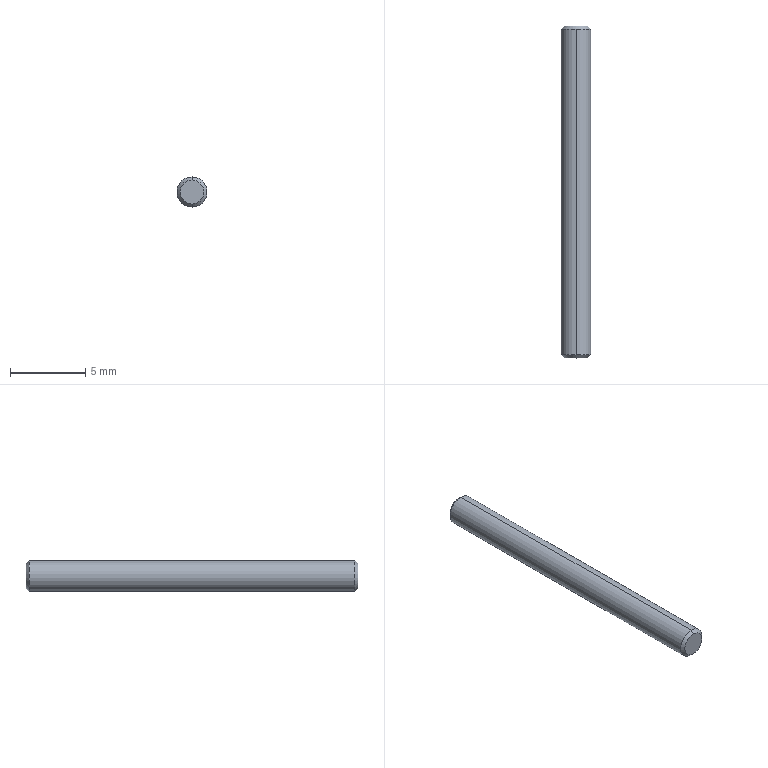Part | SolidWorks | features Chamfer 1, Extrusion 1 | 1 solid | 8 faces | box 2 x 22 x 2 mm | volume 68.88 mm3 | cone 4 | cylinder 2 | plane 2 | commonest cylinder face diameters 2 x2
STEP:
#1=CARTESIAN_POINT('',(0.,22.,0.8));
#2=VERTEX_POINT('',#1);
#3=CARTESIAN_POINT('',(0.,22.,-0.8));
#4=VERTEX_POINT('',#3);
#5=CARTESIAN_POINT('',(0.,22.,0.));
#6=DIRECTION('',(0.,1.,0.));
#7=DIRECTION('',(0.,0.,1.));
#8=AXIS2_PLACEMENT_3D('',#5,#6,#7);
#9=CIRCLE('',#8,0.8);
#10=EDGE_CURVE('',#2,#4,#9,.T.);
#11=ORIENTED_EDGE('',*,*,#10,.F.);
#12=CARTESIAN_POINT('',(0.,21.8,1.));
#13=VERTEX_POINT('',#12);
#14=CARTESIAN_POINT('',(0.,22.,0.8));
#15=DIRECTION('',(0.,-0.7071,0.7071));
#16=VECTOR('',#15,1000.);
#17=LINE('',#14,#16);
#18=EDGE_CURVE('',#2,#13,#17,.T.);
#19=ORIENTED_EDGE('',*,*,#18,.T.);
#20=CARTESIAN_POINT('',(0.,21.8,-1.));
#21=VERTEX_POINT('',#20);
#22=CARTESIAN_POINT('',(0.,21.8,0.));
#23=DIRECTION('',(0.,-1.,0.));
#24=DIRECTION('',(0.,0.,1.));
#25=AXIS2_PLACEMENT_3D('',#22,#23,#24);
#26=CIRCLE('',#25,1.);
#27=EDGE_CURVE('',#21,#13,#26,.T.);
#28=ORIENTED_EDGE('',*,*,#27,.F.);
#29=CARTESIAN_POINT('',(0.,22.,-0.8));
#30=DIRECTION('',(0.,-0.7071,-0.7071));
#31=VECTOR('',#30,1000.);
#32=LINE('',#29,#31);
#33=EDGE_CURVE('',#4,#21,#32,.T.);
#34=ORIENTED_EDGE('',*,*,#33,.F.);
#35=EDGE_LOOP('',(#11,#19,#28,#34));
#36=FACE_OUTER_BOUND('',#35,.T.);
#37=CARTESIAN_POINT('',(0.,22.,0.));
#38=DIRECTION('',(0.,-1.,0.));
#39=DIRECTION('',(0.,0.,-1.));
#40=AXIS2_PLACEMENT_3D('',#37,#38,#39);
#41=CONICAL_SURFACE('',#40,0.8,0.7854);
#42=ADVANCED_FACE('',(#36),#41,.T.);
#43=CARTESIAN_POINT('',(0.,0.,-0.8));
#44=VERTEX_POINT('',#43);
#45=CARTESIAN_POINT('',(0.,0.,0.8));
#46=VERTEX_POINT('',#45);
#47=CARTESIAN_POINT('',(0.,0.,0.));
#48=DIRECTION('',(0.,-1.,0.));
#49=DIRECTION('',(0.,0.,1.));
#50=AXIS2_PLACEMENT_3D('',#47,#48,#49);
#51=CIRCLE('',#50,0.8);
#52=EDGE_CURVE('',#44,#46,#51,.T.);
#53=ORIENTED_EDGE('',*,*,#52,.F.);
#54=CARTESIAN_POINT('',(0.,0.2,-1.));
#55=VERTEX_POINT('',#54);
#56=CARTESIAN_POINT('',(0.,0.2,-1.));
#57=DIRECTION('',(0.,0.7071,-0.7071));
#58=VECTOR('',#57,1000.);
#59=LINE('',#56,#58);
#60=EDGE_CURVE('',#44,#55,#59,.T.);
#61=ORIENTED_EDGE('',*,*,#60,.T.);
#62=CARTESIAN_POINT('',(0.,0.2,1.));
#63=VERTEX_POINT('',#62);
#64=CARTESIAN_POINT('',(0.,0.2,0.));
#65=DIRECTION('',(0.,1.,0.));
#66=DIRECTION('',(0.,0.,1.));
#67=AXIS2_PLACEMENT_3D('',#64,#65,#66);
#68=CIRCLE('',#67,1.);
#69=EDGE_CURVE('',#63,#55,#68,.T.);
#70=ORIENTED_EDGE('',*,*,#69,.F.);
#71=CARTESIAN_POINT('',(0.,0.2,1.));
#72=DIRECTION('',(0.,0.7071,0.7071));
#73=VECTOR('',#72,1000.);
#74=LINE('',#71,#73);
#75=EDGE_CURVE('',#46,#63,#74,.T.);
#76=ORIENTED_EDGE('',*,*,#75,.F.);
#77=EDGE_LOOP('',(#53,#61,#70,#76));
#78=FACE_OUTER_BOUND('',#77,.T.);
#79=CARTESIAN_POINT('',(0.,0.2,0.));
#80=DIRECTION('',(0.,1.,0.));
#81=DIRECTION('',(0.,0.,1.));
#82=AXIS2_PLACEMENT_3D('',#79,#80,#81);
#83=CONICAL_SURFACE('',#82,1.,0.7854);
#84=ADVANCED_FACE('',(#78),#83,.T.);
#85=ORIENTED_EDGE('',*,*,#27,.T.);
#86=CARTESIAN_POINT('',(0.,22.,1.));
#87=DIRECTION('',(0.,-1.,0.));
#88=VECTOR('',#87,1000.);
#89=LINE('',#86,#88);
#90=EDGE_CURVE('',#13,#63,#89,.T.);
#91=ORIENTED_EDGE('',*,*,#90,.T.);
#92=ORIENTED_EDGE('',*,*,#69,.T.);
#93=CARTESIAN_POINT('',(0.,22.,-1.));
#94=DIRECTION('',(0.,-1.,0.));
#95=VECTOR('',#94,1000.);
#96=LINE('',#93,#95);
#97=EDGE_CURVE('',#21,#55,#96,.T.);
#98=ORIENTED_EDGE('',*,*,#97,.F.);
#99=EDGE_LOOP('',(#85,#91,#92,#98));
#100=FACE_OUTER_BOUND('',#99,.T.);
#101=CARTESIAN_POINT('',(0.,22.,0.));
#102=DIRECTION('',(0.,-1.,0.));
#103=DIRECTION('',(0.,0.,-1.));
#104=AXIS2_PLACEMENT_3D('',#101,#102,#103);
#105=CYLINDRICAL_SURFACE('',#104,1.);
#106=ADVANCED_FACE('',(#100),#105,.T.);
#107=ORIENTED_EDGE('',*,*,#90,.F.);
#108=CARTESIAN_POINT('',(0.,21.8,0.));
#109=DIRECTION('',(0.,-1.,0.));
#110=DIRECTION('',(0.,0.,1.));
#111=AXIS2_PLACEMENT_3D('',#108,#109,#110);
#112=CIRCLE('',#111,1.);
#113=EDGE_CURVE('',#13,#21,#112,.T.);
#114=ORIENTED_EDGE('',*,*,#113,.T.);
#115=ORIENTED_EDGE('',*,*,#97,.T.);
#116=CARTESIAN_POINT('',(0.,0.2,0.));
#117=DIRECTION('',(0.,1.,0.));
#118=DIRECTION('',(0.,0.,1.));
#119=AXIS2_PLACEMENT_3D('',#116,#117,#118);
#120=CIRCLE('',#119,1.);
#121=EDGE_CURVE('',#55,#63,#120,.T.);
#122=ORIENTED_EDGE('',*,*,#121,.T.);
#123=EDGE_LOOP('',(#107,#114,#115,#122));
#124=FACE_OUTER_BOUND('',#123,.T.);
#125=CARTESIAN_POINT('',(0.,22.,0.));
#126=DIRECTION('',(0.,-1.,0.));
#127=DIRECTION('',(0.,0.,-1.));
#128=AXIS2_PLACEMENT_3D('',#125,#126,#127);
#129=CYLINDRICAL_SURFACE('',#128,1.);
#130=ADVANCED_FACE('',(#124),#129,.T.);
#131=CARTESIAN_POINT('',(0.,22.,0.));
#132=DIRECTION('',(0.,1.,0.));
#133=DIRECTION('',(0.,0.,1.));
#134=AXIS2_PLACEMENT_3D('',#131,#132,#133);
#135=CIRCLE('',#134,0.8);
#136=EDGE_CURVE('',#4,#2,#135,.T.);
#137=ORIENTED_EDGE('',*,*,#136,.T.);
#138=ORIENTED_EDGE('',*,*,#10,.T.);
#139=EDGE_LOOP('',(#137,#138));
#140=FACE_OUTER_BOUND('',#139,.T.);
#141=CARTESIAN_POINT('',(0.,22.,0.));
#142=DIRECTION('',(0.,1.,0.));
#143=DIRECTION('',(0.,0.,1.));
#144=AXIS2_PLACEMENT_3D('',#141,#142,#143);
#145=PLANE('',#144);
#146=ADVANCED_FACE('',(#140),#145,.T.);
#147=CARTESIAN_POINT('',(0.,0.,0.));
#148=DIRECTION('',(0.,-1.,0.));
#149=DIRECTION('',(0.,0.,1.));
#150=AXIS2_PLACEMENT_3D('',#147,#148,#149);
#151=CIRCLE('',#150,0.8);
#152=EDGE_CURVE('',#46,#44,#151,.T.);
#153=ORIENTED_EDGE('',*,*,#152,.T.);
#154=ORIENTED_EDGE('',*,*,#52,.T.);
#155=EDGE_LOOP('',(#153,#154));
#156=FACE_OUTER_BOUND('',#155,.T.);
#157=CARTESIAN_POINT('',(0.,0.,0.));
#158=DIRECTION('',(0.,1.,0.));
#159=DIRECTION('',(0.,0.,1.));
#160=AXIS2_PLACEMENT_3D('',#157,#158,#159);
#161=PLANE('',#160);
#162=ADVANCED_FACE('',(#156),#161,.F.);
#163=ORIENTED_EDGE('',*,*,#60,.F.);
#164=ORIENTED_EDGE('',*,*,#152,.F.);
#165=ORIENTED_EDGE('',*,*,#75,.T.);
#166=ORIENTED_EDGE('',*,*,#121,.F.);
#167=EDGE_LOOP('',(#163,#164,#165,#166));
#168=FACE_OUTER_BOUND('',#167,.T.);
#169=CARTESIAN_POINT('',(0.,0.2,0.));
#170=DIRECTION('',(0.,1.,0.));
#171=DIRECTION('',(0.,0.,1.));
#172=AXIS2_PLACEMENT_3D('',#169,#170,#171);
#173=CONICAL_SURFACE('',#172,1.,0.7854);
#174=ADVANCED_FACE('',(#168),#173,.T.);
#175=ORIENTED_EDGE('',*,*,#18,.F.);
#176=ORIENTED_EDGE('',*,*,#136,.F.);
#177=ORIENTED_EDGE('',*,*,#33,.T.);
#178=ORIENTED_EDGE('',*,*,#113,.F.);
#179=EDGE_LOOP('',(#175,#176,#177,#178));
#180=FACE_OUTER_BOUND('',#179,.T.);
#181=CARTESIAN_POINT('',(0.,22.,0.));
#182=DIRECTION('',(0.,-1.,0.));
#183=DIRECTION('',(0.,0.,-1.));
#184=AXIS2_PLACEMENT_3D('',#181,#182,#183);
#185=CONICAL_SURFACE('',#184,0.8,0.7854);
#186=ADVANCED_FACE('',(#180),#185,.T.);
#187=CLOSED_SHELL('',(#42,#84,#106,#130,#146,#162,#174,#186));
#188=MANIFOLD_SOLID_BREP('',#187);
#189=CARTESIAN_POINT('',(0.,0.,0.));
#190=DIRECTION('',(0.,0.,1.));
#191=DIRECTION('',(1.,0.,0.));
#192=AXIS2_PLACEMENT_3D('',#189,#190,#191);
#193=(LENGTH_UNIT()NAMED_UNIT(*)SI_UNIT(.MILLI.,.METRE.));
#194=UNCERTAINTY_MEASURE_WITH_UNIT(LENGTH_MEASURE(0.00001),#193,'','');
#195=(NAMED_UNIT(*)PLANE_ANGLE_UNIT()SI_UNIT($,.RADIAN.));
#196=(NAMED_UNIT(*)SI_UNIT($,.STERADIAN.)SOLID_ANGLE_UNIT());
#197=(GEOMETRIC_REPRESENTATION_CONTEXT(3)GLOBAL_UNCERTAINTY_ASSIGNED_CONTEXT((#194))GLOBAL_UNIT_ASSIGNED_CONTEXT((#193,#195,#196))REPRESENTATION_CONTEXT('',''));
#198=ADVANCED_BREP_SHAPE_REPRESENTATION('',(#188,#192),#197);